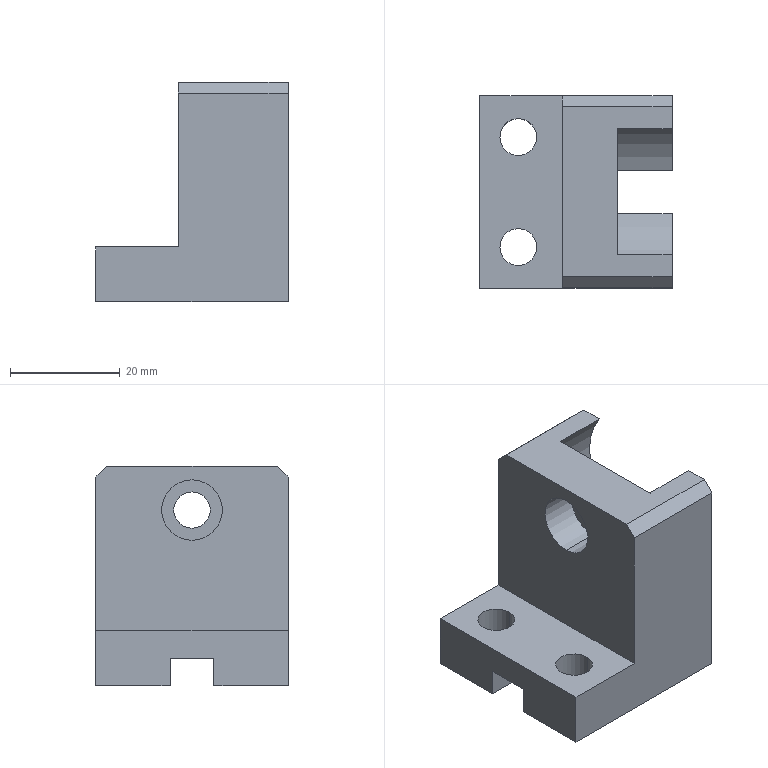Part | STEP file | Part 1^Dual platform unit | 1 solid | 27 faces | box 35 x 35 x 40 mm | volume 24064 mm3 | plane 17 | cylinder 10 | commonest cylinder face diameters 6.7 x4 6.6 x2 11 x2 28 x2
STEP:
#1=CARTESIAN_POINT('',(-416.35,-17.5,0.));
#2=VERTEX_POINT('',#1);
#3=CARTESIAN_POINT('',(-409.65,-17.5,0.));
#4=VERTEX_POINT('',#3);
#5=CARTESIAN_POINT('',(-413.,-17.5,0.));
#6=DIRECTION('',(0.,0.,1.));
#7=DIRECTION('',(1.,0.,0.));
#8=AXIS2_PLACEMENT_3D('',#5,#6,#7);
#9=CIRCLE('',#8,3.35);
#10=EDGE_CURVE('',#2,#4,#9,.T.);
#11=ORIENTED_EDGE('',*,*,#10,.F.);
#12=CARTESIAN_POINT('',(-416.35,-17.5,10.));
#13=VERTEX_POINT('',#12);
#14=CARTESIAN_POINT('',(-416.35,-17.5,10.));
#15=DIRECTION('',(0.,0.,1.));
#16=VECTOR('',#15,1000.);
#17=LINE('',#14,#16);
#18=EDGE_CURVE('',#2,#13,#17,.T.);
#19=ORIENTED_EDGE('',*,*,#18,.T.);
#20=CARTESIAN_POINT('',(-409.65,-17.5,10.));
#21=VERTEX_POINT('',#20);
#22=CARTESIAN_POINT('',(-413.,-17.5,10.));
#23=DIRECTION('',(0.,0.,1.));
#24=DIRECTION('',(1.,0.,0.));
#25=AXIS2_PLACEMENT_3D('',#22,#23,#24);
#26=CIRCLE('',#25,3.35);
#27=EDGE_CURVE('',#13,#21,#26,.T.);
#28=ORIENTED_EDGE('',*,*,#27,.T.);
#29=CARTESIAN_POINT('',(-409.65,-17.5,10.));
#30=DIRECTION('',(0.,0.,1.));
#31=VECTOR('',#30,1000.);
#32=LINE('',#29,#31);
#33=EDGE_CURVE('',#4,#21,#32,.T.);
#34=ORIENTED_EDGE('',*,*,#33,.F.);
#35=EDGE_LOOP('',(#11,#19,#28,#34));
#36=FACE_OUTER_BOUND('',#35,.T.);
#37=CARTESIAN_POINT('',(-413.,-17.5,10.));
#38=DIRECTION('',(0.,0.,1.));
#39=DIRECTION('',(1.,0.,0.));
#40=AXIS2_PLACEMENT_3D('',#37,#38,#39);
#41=CYLINDRICAL_SURFACE('',#40,3.35);
#42=ADVANCED_FACE('',(#36),#41,.F.);
#43=CARTESIAN_POINT('',(-416.35,-37.5,0.));
#44=VERTEX_POINT('',#43);
#45=CARTESIAN_POINT('',(-409.65,-37.5,0.));
#46=VERTEX_POINT('',#45);
#47=CARTESIAN_POINT('',(-413.,-37.5,0.));
#48=DIRECTION('',(0.,0.,1.));
#49=DIRECTION('',(1.,0.,0.));
#50=AXIS2_PLACEMENT_3D('',#47,#48,#49);
#51=CIRCLE('',#50,3.35);
#52=EDGE_CURVE('',#44,#46,#51,.T.);
#53=ORIENTED_EDGE('',*,*,#52,.F.);
#54=CARTESIAN_POINT('',(-416.35,-37.5,10.));
#55=VERTEX_POINT('',#54);
#56=CARTESIAN_POINT('',(-416.35,-37.5,10.));
#57=DIRECTION('',(0.,0.,1.));
#58=VECTOR('',#57,1000.);
#59=LINE('',#56,#58);
#60=EDGE_CURVE('',#44,#55,#59,.T.);
#61=ORIENTED_EDGE('',*,*,#60,.T.);
#62=CARTESIAN_POINT('',(-409.65,-37.5,10.));
#63=VERTEX_POINT('',#62);
#64=CARTESIAN_POINT('',(-413.,-37.5,10.));
#65=DIRECTION('',(0.,0.,1.));
#66=DIRECTION('',(1.,0.,0.));
#67=AXIS2_PLACEMENT_3D('',#64,#65,#66);
#68=CIRCLE('',#67,3.35);
#69=EDGE_CURVE('',#55,#63,#68,.T.);
#70=ORIENTED_EDGE('',*,*,#69,.T.);
#71=CARTESIAN_POINT('',(-409.65,-37.5,10.));
#72=DIRECTION('',(0.,0.,1.));
#73=VECTOR('',#72,1000.);
#74=LINE('',#71,#73);
#75=EDGE_CURVE('',#46,#63,#74,.T.);
#76=ORIENTED_EDGE('',*,*,#75,.F.);
#77=EDGE_LOOP('',(#53,#61,#70,#76));
#78=FACE_OUTER_BOUND('',#77,.T.);
#79=CARTESIAN_POINT('',(-413.,-37.5,10.));
#80=DIRECTION('',(0.,0.,1.));
#81=DIRECTION('',(1.,0.,0.));
#82=AXIS2_PLACEMENT_3D('',#79,#80,#81);
#83=CYLINDRICAL_SURFACE('',#82,3.35);
#84=ADVANCED_FACE('',(#78),#83,.F.);
#85=CARTESIAN_POINT('',(-398.2,-27.5,26.5));
#86=VERTEX_POINT('',#85);
#87=CARTESIAN_POINT('',(-398.2,-27.5,37.5));
#88=VERTEX_POINT('',#87);
#89=CARTESIAN_POINT('',(-398.2,-27.5,32.));
#90=DIRECTION('',(-1.,0.,0.));
#91=DIRECTION('',(0.,0.,1.));
#92=AXIS2_PLACEMENT_3D('',#89,#90,#91);
#93=CIRCLE('',#92,5.5);
#94=EDGE_CURVE('',#86,#88,#93,.T.);
#95=ORIENTED_EDGE('',*,*,#94,.F.);
#96=CARTESIAN_POINT('',(-405.,-27.5,26.5));
#97=VERTEX_POINT('',#96);
#98=CARTESIAN_POINT('',(-405.,-27.5,26.5));
#99=DIRECTION('',(-1.,0.,0.));
#100=VECTOR('',#99,1000.);
#101=LINE('',#98,#100);
#102=EDGE_CURVE('',#86,#97,#101,.T.);
#103=ORIENTED_EDGE('',*,*,#102,.T.);
#104=CARTESIAN_POINT('',(-405.,-27.5,37.5));
#105=VERTEX_POINT('',#104);
#106=CARTESIAN_POINT('',(-405.,-27.5,32.));
#107=DIRECTION('',(-1.,0.,0.));
#108=DIRECTION('',(0.,0.,1.));
#109=AXIS2_PLACEMENT_3D('',#106,#107,#108);
#110=CIRCLE('',#109,5.5);
#111=EDGE_CURVE('',#97,#105,#110,.T.);
#112=ORIENTED_EDGE('',*,*,#111,.T.);
#113=CARTESIAN_POINT('',(-405.,-27.5,37.5));
#114=DIRECTION('',(-1.,0.,0.));
#115=VECTOR('',#114,1000.);
#116=LINE('',#113,#115);
#117=EDGE_CURVE('',#88,#105,#116,.T.);
#118=ORIENTED_EDGE('',*,*,#117,.F.);
#119=EDGE_LOOP('',(#95,#103,#112,#118));
#120=FACE_OUTER_BOUND('',#119,.T.);
#121=CARTESIAN_POINT('',(-405.,-27.5,32.));
#122=DIRECTION('',(-1.,0.,0.));
#123=DIRECTION('',(0.,0.,1.));
#124=AXIS2_PLACEMENT_3D('',#121,#122,#123);
#125=CYLINDRICAL_SURFACE('',#124,5.5);
#126=ADVANCED_FACE('',(#120),#125,.F.);
#127=CARTESIAN_POINT('',(-395.,-27.5,35.3));
#128=VERTEX_POINT('',#127);
#129=CARTESIAN_POINT('',(-395.,-27.5,28.7));
#130=VERTEX_POINT('',#129);
#131=CARTESIAN_POINT('',(-395.,-27.5,32.));
#132=DIRECTION('',(1.,0.,0.));
#133=DIRECTION('',(0.,0.,-1.));
#134=AXIS2_PLACEMENT_3D('',#131,#132,#133);
#135=CIRCLE('',#134,3.3);
#136=EDGE_CURVE('',#128,#130,#135,.T.);
#137=ORIENTED_EDGE('',*,*,#136,.T.);
#138=CARTESIAN_POINT('',(-398.2,-27.5,28.7));
#139=VERTEX_POINT('',#138);
#140=CARTESIAN_POINT('',(-405.,-27.5,28.7));
#141=DIRECTION('',(-1.,0.,0.));
#142=VECTOR('',#141,1000.);
#143=LINE('',#140,#142);
#144=EDGE_CURVE('',#130,#139,#143,.T.);
#145=ORIENTED_EDGE('',*,*,#144,.T.);
#146=CARTESIAN_POINT('',(-398.2,-27.5,35.3));
#147=VERTEX_POINT('',#146);
#148=CARTESIAN_POINT('',(-398.2,-27.5,32.));
#149=DIRECTION('',(-1.,0.,0.));
#150=DIRECTION('',(0.,0.,1.));
#151=AXIS2_PLACEMENT_3D('',#148,#149,#150);
#152=CIRCLE('',#151,3.3);
#153=EDGE_CURVE('',#139,#147,#152,.T.);
#154=ORIENTED_EDGE('',*,*,#153,.T.);
#155=CARTESIAN_POINT('',(-405.,-27.5,35.3));
#156=DIRECTION('',(-1.,0.,0.));
#157=VECTOR('',#156,1000.);
#158=LINE('',#155,#157);
#159=EDGE_CURVE('',#128,#147,#158,.T.);
#160=ORIENTED_EDGE('',*,*,#159,.F.);
#161=EDGE_LOOP('',(#137,#145,#154,#160));
#162=FACE_OUTER_BOUND('',#161,.T.);
#163=CARTESIAN_POINT('',(-405.,-27.5,32.));
#164=DIRECTION('',(-1.,0.,0.));
#165=DIRECTION('',(0.,0.,1.));
#166=AXIS2_PLACEMENT_3D('',#163,#164,#165);
#167=CYLINDRICAL_SURFACE('',#166,3.3);
#168=ADVANCED_FACE('',(#162),#167,.F.);
#169=CARTESIAN_POINT('',(-413.,-37.5,0.));
#170=DIRECTION('',(0.,0.,1.));
#171=DIRECTION('',(1.,0.,0.));
#172=AXIS2_PLACEMENT_3D('',#169,#170,#171);
#173=CIRCLE('',#172,3.35);
#174=EDGE_CURVE('',#46,#44,#173,.T.);
#175=ORIENTED_EDGE('',*,*,#174,.T.);
#176=ORIENTED_EDGE('',*,*,#52,.T.);
#177=EDGE_LOOP('',(#175,#176));
#178=FACE_BOUND('',#177,.T.);
#179=CARTESIAN_POINT('',(-420.,-31.5,0.));
#180=VERTEX_POINT('',#179);
#181=CARTESIAN_POINT('',(-420.,-45.,0.));
#182=VERTEX_POINT('',#181);
#183=CARTESIAN_POINT('',(-420.,-45.,0.));
#184=DIRECTION('',(0.,-1.,0.));
#185=VECTOR('',#184,1000.);
#186=LINE('',#183,#185);
#187=EDGE_CURVE('',#180,#182,#186,.T.);
#188=ORIENTED_EDGE('',*,*,#187,.F.);
#189=CARTESIAN_POINT('',(-385.,-31.5,0.));
#190=VERTEX_POINT('',#189);
#191=CARTESIAN_POINT('',(-395.,-31.5,0.));
#192=DIRECTION('',(1.,0.,0.));
#193=VECTOR('',#192,1000.);
#194=LINE('',#191,#193);
#195=EDGE_CURVE('',#180,#190,#194,.T.);
#196=ORIENTED_EDGE('',*,*,#195,.T.);
#197=CARTESIAN_POINT('',(-385.,-45.,0.));
#198=VERTEX_POINT('',#197);
#199=CARTESIAN_POINT('',(-385.,-45.,0.));
#200=DIRECTION('',(0.,1.,0.));
#201=VECTOR('',#200,1000.);
#202=LINE('',#199,#201);
#203=EDGE_CURVE('',#198,#190,#202,.T.);
#204=ORIENTED_EDGE('',*,*,#203,.F.);
#205=CARTESIAN_POINT('',(-385.,-45.,0.));
#206=DIRECTION('',(1.,0.,0.));
#207=VECTOR('',#206,1000.);
#208=LINE('',#205,#207);
#209=EDGE_CURVE('',#182,#198,#208,.T.);
#210=ORIENTED_EDGE('',*,*,#209,.F.);
#211=EDGE_LOOP('',(#188,#196,#204,#210));
#212=FACE_OUTER_BOUND('',#211,.T.);
#213=CARTESIAN_POINT('',(0.,0.,0.));
#214=DIRECTION('',(0.,0.,1.));
#215=DIRECTION('',(1.,0.,0.));
#216=AXIS2_PLACEMENT_3D('',#213,#214,#215);
#217=PLANE('',#216);
#218=ADVANCED_FACE('',(#178,#212),#217,.F.);
#219=CARTESIAN_POINT('',(-385.,-43.,40.));
#220=VERTEX_POINT('',#219);
#221=CARTESIAN_POINT('',(-385.,-38.989,40.));
#222=VERTEX_POINT('',#221);
#223=CARTESIAN_POINT('',(-385.,-45.,40.));
#224=DIRECTION('',(0.,1.,0.));
#225=VECTOR('',#224,1000.);
#226=LINE('',#223,#225);
#227=EDGE_CURVE('',#220,#222,#226,.T.);
#228=ORIENTED_EDGE('',*,*,#227,.F.);
#229=CARTESIAN_POINT('',(-385.,-45.,38.));
#230=VERTEX_POINT('',#229);
#231=CARTESIAN_POINT('',(-385.,-43.,40.));
#232=DIRECTION('',(0.,-0.7071,-0.7071));
#233=VECTOR('',#232,1000.);
#234=LINE('',#231,#233);
#235=EDGE_CURVE('',#220,#230,#234,.T.);
#236=ORIENTED_EDGE('',*,*,#235,.T.);
#237=CARTESIAN_POINT('',(-385.,-45.,40.));
#238=DIRECTION('',(0.,0.,-1.));
#239=VECTOR('',#238,1000.);
#240=LINE('',#237,#239);
#241=EDGE_CURVE('',#230,#198,#240,.T.);
#242=ORIENTED_EDGE('',*,*,#241,.T.);
#243=ORIENTED_EDGE('',*,*,#203,.T.);
#244=CARTESIAN_POINT('',(-385.,-31.5,18.584));
#245=VERTEX_POINT('',#244);
#246=CARTESIAN_POINT('',(-385.,-31.5,0.));
#247=DIRECTION('',(0.,0.,-1.));
#248=VECTOR('',#247,1000.);
#249=LINE('',#246,#248);
#250=EDGE_CURVE('',#245,#190,#249,.T.);
#251=ORIENTED_EDGE('',*,*,#250,.F.);
#252=CARTESIAN_POINT('',(-385.,-27.5,32.));
#253=DIRECTION('',(1.,0.,0.));
#254=DIRECTION('',(0.,0.,-1.));
#255=AXIS2_PLACEMENT_3D('',#252,#253,#254);
#256=CIRCLE('',#255,14.);
#257=EDGE_CURVE('',#222,#245,#256,.T.);
#258=ORIENTED_EDGE('',*,*,#257,.F.);
#259=EDGE_LOOP('',(#228,#236,#242,#243,#251,#258));
#260=FACE_OUTER_BOUND('',#259,.T.);
#261=CARTESIAN_POINT('',(-385.,-45.,40.));
#262=DIRECTION('',(-1.,0.,0.));
#263=DIRECTION('',(0.,0.,1.));
#264=AXIS2_PLACEMENT_3D('',#261,#262,#263);
#265=PLANE('',#264);
#266=ADVANCED_FACE('',(#260),#265,.F.);
#267=ORIENTED_EDGE('',*,*,#257,.T.);
#268=CARTESIAN_POINT('',(-395.,-31.5,18.584));
#269=VERTEX_POINT('',#268);
#270=CARTESIAN_POINT('',(-395.,-31.5,18.584));
#271=DIRECTION('',(-1.,0.,0.));
#272=VECTOR('',#271,1000.);
#273=LINE('',#270,#272);
#274=EDGE_CURVE('',#245,#269,#273,.T.);
#275=ORIENTED_EDGE('',*,*,#274,.T.);
#276=CARTESIAN_POINT('',(-395.,-38.989,40.));
#277=VERTEX_POINT('',#276);
#278=CARTESIAN_POINT('',(-395.,-27.5,32.));
#279=DIRECTION('',(1.,0.,0.));
#280=DIRECTION('',(0.,0.,-1.));
#281=AXIS2_PLACEMENT_3D('',#278,#279,#280);
#282=CIRCLE('',#281,14.);
#283=EDGE_CURVE('',#277,#269,#282,.T.);
#284=ORIENTED_EDGE('',*,*,#283,.F.);
#285=CARTESIAN_POINT('',(-395.,-38.989,40.));
#286=DIRECTION('',(1.,0.,0.));
#287=VECTOR('',#286,1000.);
#288=LINE('',#285,#287);
#289=EDGE_CURVE('',#277,#222,#288,.T.);
#290=ORIENTED_EDGE('',*,*,#289,.T.);
#291=EDGE_LOOP('',(#267,#275,#284,#290));
#292=FACE_OUTER_BOUND('',#291,.T.);
#293=CARTESIAN_POINT('',(-395.,-27.5,32.));
#294=DIRECTION('',(1.,0.,0.));
#295=DIRECTION('',(0.,0.,-1.));
#296=AXIS2_PLACEMENT_3D('',#293,#294,#295);
#297=CYLINDRICAL_SURFACE('',#296,14.);
#298=ADVANCED_FACE('',(#292),#297,.F.);
#299=CARTESIAN_POINT('',(-385.,-10.,38.));
#300=VERTEX_POINT('',#299);
#301=CARTESIAN_POINT('',(-385.,-10.,0.));
#302=VERTEX_POINT('',#301);
#303=CARTESIAN_POINT('',(-385.,-10.,40.));
#304=DIRECTION('',(0.,0.,-1.));
#305=VECTOR('',#304,1000.);
#306=LINE('',#303,#305);
#307=EDGE_CURVE('',#300,#302,#306,.T.);
#308=ORIENTED_EDGE('',*,*,#307,.F.);
#309=CARTESIAN_POINT('',(-385.,-12.,40.));
#310=VERTEX_POINT('',#309);
#311=CARTESIAN_POINT('',(-385.,-12.,40.));
#312=DIRECTION('',(0.,-0.7071,0.7071));
#313=VECTOR('',#312,1000.);
#314=LINE('',#311,#313);
#315=EDGE_CURVE('',#300,#310,#314,.T.);
#316=ORIENTED_EDGE('',*,*,#315,.T.);
#317=CARTESIAN_POINT('',(-385.,-16.011,40.));
#318=VERTEX_POINT('',#317);
#319=CARTESIAN_POINT('',(-385.,-45.,40.));
#320=DIRECTION('',(0.,1.,0.));
#321=VECTOR('',#320,1000.);
#322=LINE('',#319,#321);
#323=EDGE_CURVE('',#318,#310,#322,.T.);
#324=ORIENTED_EDGE('',*,*,#323,.F.);
#325=CARTESIAN_POINT('',(-385.,-23.5,18.584));
#326=VERTEX_POINT('',#325);
#327=CARTESIAN_POINT('',(-385.,-27.5,32.));
#328=DIRECTION('',(1.,0.,0.));
#329=DIRECTION('',(0.,0.,-1.));
#330=AXIS2_PLACEMENT_3D('',#327,#328,#329);
#331=CIRCLE('',#330,14.);
#332=EDGE_CURVE('',#326,#318,#331,.T.);
#333=ORIENTED_EDGE('',*,*,#332,.F.);
#334=CARTESIAN_POINT('',(-385.,-23.5,0.));
#335=VERTEX_POINT('',#334);
#336=CARTESIAN_POINT('',(-385.,-23.5,0.));
#337=DIRECTION('',(0.,0.,1.));
#338=VECTOR('',#337,1000.);
#339=LINE('',#336,#338);
#340=EDGE_CURVE('',#335,#326,#339,.T.);
#341=ORIENTED_EDGE('',*,*,#340,.F.);
#342=CARTESIAN_POINT('',(-385.,-45.,0.));
#343=DIRECTION('',(0.,1.,0.));
#344=VECTOR('',#343,1000.);
#345=LINE('',#342,#344);
#346=EDGE_CURVE('',#335,#302,#345,.T.);
#347=ORIENTED_EDGE('',*,*,#346,.T.);
#348=EDGE_LOOP('',(#308,#316,#324,#333,#341,#347));
#349=FACE_OUTER_BOUND('',#348,.T.);
#350=CARTESIAN_POINT('',(-385.,-45.,40.));
#351=DIRECTION('',(-1.,0.,0.));
#352=DIRECTION('',(0.,0.,1.));
#353=AXIS2_PLACEMENT_3D('',#350,#351,#352);
#354=PLANE('',#353);
#355=ADVANCED_FACE('',(#349),#354,.F.);
#356=CARTESIAN_POINT('',(-405.,-10.,38.));
#357=VERTEX_POINT('',#356);
#358=CARTESIAN_POINT('',(-405.,-10.,10.));
#359=VERTEX_POINT('',#358);
#360=CARTESIAN_POINT('',(-405.,-10.,40.));
#361=DIRECTION('',(0.,0.,-1.));
#362=VECTOR('',#361,1000.);
#363=LINE('',#360,#362);
#364=EDGE_CURVE('',#357,#359,#363,.T.);
#365=ORIENTED_EDGE('',*,*,#364,.F.);
#366=CARTESIAN_POINT('',(-385.,-10.,38.));
#367=DIRECTION('',(1.,0.,0.));
#368=VECTOR('',#367,1000.);
#369=LINE('',#366,#368);
#370=EDGE_CURVE('',#357,#300,#369,.T.);
#371=ORIENTED_EDGE('',*,*,#370,.T.);
#372=ORIENTED_EDGE('',*,*,#307,.T.);
#373=CARTESIAN_POINT('',(-420.,-10.,0.));
#374=VERTEX_POINT('',#373);
#375=CARTESIAN_POINT('',(-385.,-10.,0.));
#376=DIRECTION('',(-1.,0.,0.));
#377=VECTOR('',#376,1000.);
#378=LINE('',#375,#377);
#379=EDGE_CURVE('',#302,#374,#378,.T.);
#380=ORIENTED_EDGE('',*,*,#379,.T.);
#381=CARTESIAN_POINT('',(-420.,-10.,10.));
#382=VERTEX_POINT('',#381);
#383=CARTESIAN_POINT('',(-420.,-10.,40.));
#384=DIRECTION('',(0.,0.,-1.));
#385=VECTOR('',#384,1000.);
#386=LINE('',#383,#385);
#387=EDGE_CURVE('',#382,#374,#386,.T.);
#388=ORIENTED_EDGE('',*,*,#387,.F.);
#389=CARTESIAN_POINT('',(-405.,-10.,10.));
#390=DIRECTION('',(-1.,0.,0.));
#391=VECTOR('',#390,1000.);
#392=LINE('',#389,#391);
#393=EDGE_CURVE('',#359,#382,#392,.T.);
#394=ORIENTED_EDGE('',*,*,#393,.F.);
#395=EDGE_LOOP('',(#365,#371,#372,#380,#388,#394));
#396=FACE_OUTER_BOUND('',#395,.T.);
#397=CARTESIAN_POINT('',(-385.,-10.,40.));
#398=DIRECTION('',(0.,-1.,0.));
#399=DIRECTION('',(1.,0.,0.));
#400=AXIS2_PLACEMENT_3D('',#397,#398,#399);
#401=PLANE('',#400);
#402=ADVANCED_FACE('',(#396),#401,.F.);
#403=CARTESIAN_POINT('',(-420.,-31.5,5.));
#404=VERTEX_POINT('',#403);
#405=CARTESIAN_POINT('',(-420.,-23.5,5.));
#406=VERTEX_POINT('',#405);
#407=CARTESIAN_POINT('',(-420.,-23.5,5.));
#408=DIRECTION('',(0.,1.,0.));
#409=VECTOR('',#408,1000.);
#410=LINE('',#407,#409);
#411=EDGE_CURVE('',#404,#406,#410,.T.);
#412=ORIENTED_EDGE('',*,*,#411,.F.);
#413=CARTESIAN_POINT('',(-420.,-31.5,5.));
#414=DIRECTION('',(0.,0.,-1.));
#415=VECTOR('',#414,1000.);
#416=LINE('',#413,#415);
#417=EDGE_CURVE('',#404,#180,#416,.T.);
#418=ORIENTED_EDGE('',*,*,#417,.T.);
#419=ORIENTED_EDGE('',*,*,#187,.T.);
#420=CARTESIAN_POINT('',(-420.,-45.,10.));
#421=VERTEX_POINT('',#420);
#422=CARTESIAN_POINT('',(-420.,-45.,40.));
#423=DIRECTION('',(0.,0.,-1.));
#424=VECTOR('',#423,1000.);
#425=LINE('',#422,#424);
#426=EDGE_CURVE('',#421,#182,#425,.T.);
#427=ORIENTED_EDGE('',*,*,#426,.F.);
#428=CARTESIAN_POINT('',(-420.,-10.,10.));
#429=DIRECTION('',(0.,-1.,0.));
#430=VECTOR('',#429,1000.);
#431=LINE('',#428,#430);
#432=EDGE_CURVE('',#382,#421,#431,.T.);
#433=ORIENTED_EDGE('',*,*,#432,.F.);
#434=ORIENTED_EDGE('',*,*,#387,.T.);
#435=CARTESIAN_POINT('',(-420.,-23.5,0.));
#436=VERTEX_POINT('',#435);
#437=CARTESIAN_POINT('',(-420.,-45.,0.));
#438=DIRECTION('',(0.,-1.,0.));
#439=VECTOR('',#438,1000.);
#440=LINE('',#437,#439);
#441=EDGE_CURVE('',#374,#436,#440,.T.);
#442=ORIENTED_EDGE('',*,*,#441,.T.);
#443=CARTESIAN_POINT('',(-420.,-23.5,5.));
#444=DIRECTION('',(0.,0.,-1.));
#445=VECTOR('',#444,1000.);
#446=LINE('',#443,#445);
#447=EDGE_CURVE('',#406,#436,#446,.T.);
#448=ORIENTED_EDGE('',*,*,#447,.F.);
#449=EDGE_LOOP('',(#412,#418,#419,#427,#433,#434,#442,#448));
#450=FACE_OUTER_BOUND('',#449,.T.);
#451=CARTESIAN_POINT('',(-420.,-45.,40.));
#452=DIRECTION('',(1.,0.,0.));
#453=DIRECTION('',(0.,0.,-1.));
#454=AXIS2_PLACEMENT_3D('',#451,#452,#453);
#455=PLANE('',#454);
#456=ADVANCED_FACE('',(#450),#455,.F.);
#457=ORIENTED_EDGE('',*,*,#241,.F.);
#458=CARTESIAN_POINT('',(-405.,-45.,38.));
#459=VERTEX_POINT('',#458);
#460=CARTESIAN_POINT('',(-405.,-45.,38.));
#461=DIRECTION('',(-1.,0.,0.));
#462=VECTOR('',#461,1000.);
#463=LINE('',#460,#462);
#464=EDGE_CURVE('',#230,#459,#463,.T.);
#465=ORIENTED_EDGE('',*,*,#464,.T.);
#466=CARTESIAN_POINT('',(-405.,-45.,10.));
#467=VERTEX_POINT('',#466);
#468=CARTESIAN_POINT('',(-405.,-45.,40.));
#469=DIRECTION('',(0.,0.,1.));
#470=VECTOR('',#469,1000.);
#471=LINE('',#468,#470);
#472=EDGE_CURVE('',#467,#459,#471,.T.);
#473=ORIENTED_EDGE('',*,*,#472,.F.);
#474=CARTESIAN_POINT('',(-405.,-45.,10.));
#475=DIRECTION('',(-1.,0.,0.));
#476=VECTOR('',#475,1000.);
#477=LINE('',#474,#476);
#478=EDGE_CURVE('',#467,#421,#477,.T.);
#479=ORIENTED_EDGE('',*,*,#478,.T.);
#480=ORIENTED_EDGE('',*,*,#426,.T.);
#481=ORIENTED_EDGE('',*,*,#209,.T.);
#482=EDGE_LOOP('',(#457,#465,#473,#479,#480,#481));
#483=FACE_OUTER_BOUND('',#482,.T.);
#484=CARTESIAN_POINT('',(-385.,-45.,40.));
#485=DIRECTION('',(0.,1.,0.));
#486=DIRECTION('',(0.,0.,1.));
#487=AXIS2_PLACEMENT_3D('',#484,#485,#486);
#488=PLANE('',#487);
#489=ADVANCED_FACE('',(#483),#488,.F.);
#490=ORIENTED_EDGE('',*,*,#323,.T.);
#491=CARTESIAN_POINT('',(-405.,-12.,40.));
#492=VERTEX_POINT('',#491);
#493=CARTESIAN_POINT('',(-405.,-12.,40.));
#494=DIRECTION('',(-1.,0.,0.));
#495=VECTOR('',#494,1000.);
#496=LINE('',#493,#495);
#497=EDGE_CURVE('',#310,#492,#496,.T.);
#498=ORIENTED_EDGE('',*,*,#497,.T.);
#499=CARTESIAN_POINT('',(-405.,-43.,40.));
#500=VERTEX_POINT('',#499);
#501=CARTESIAN_POINT('',(-405.,-10.,40.));
#502=DIRECTION('',(0.,1.,0.));
#503=VECTOR('',#502,1000.);
#504=LINE('',#501,#503);
#505=EDGE_CURVE('',#500,#492,#504,.T.);
#506=ORIENTED_EDGE('',*,*,#505,.F.);
#507=CARTESIAN_POINT('',(-385.,-43.,40.));
#508=DIRECTION('',(1.,0.,0.));
#509=VECTOR('',#508,1000.);
#510=LINE('',#507,#509);
#511=EDGE_CURVE('',#500,#220,#510,.T.);
#512=ORIENTED_EDGE('',*,*,#511,.T.);
#513=ORIENTED_EDGE('',*,*,#227,.T.);
#514=ORIENTED_EDGE('',*,*,#289,.F.);
#515=CARTESIAN_POINT('',(-395.,-16.011,40.));
#516=VERTEX_POINT('',#515);
#517=CARTESIAN_POINT('',(-395.,0.,40.));
#518=DIRECTION('',(0.,1.,0.));
#519=VECTOR('',#518,1000.);
#520=LINE('',#517,#519);
#521=EDGE_CURVE('',#277,#516,#520,.T.);
#522=ORIENTED_EDGE('',*,*,#521,.T.);
#523=CARTESIAN_POINT('',(-395.,-16.011,40.));
#524=DIRECTION('',(-1.,0.,0.));
#525=VECTOR('',#524,1000.);
#526=LINE('',#523,#525);
#527=EDGE_CURVE('',#318,#516,#526,.T.);
#528=ORIENTED_EDGE('',*,*,#527,.F.);
#529=EDGE_LOOP('',(#490,#498,#506,#512,#513,#514,#522,#528));
#530=FACE_OUTER_BOUND('',#529,.T.);
#531=CARTESIAN_POINT('',(0.,0.,40.));
#532=DIRECTION('',(0.,0.,1.));
#533=DIRECTION('',(1.,0.,0.));
#534=AXIS2_PLACEMENT_3D('',#531,#532,#533);
#535=PLANE('',#534);
#536=ADVANCED_FACE('',(#530),#535,.T.);
#537=CARTESIAN_POINT('',(-413.,-17.5,0.));
#538=DIRECTION('',(0.,0.,1.));
#539=DIRECTION('',(1.,0.,0.));
#540=AXIS2_PLACEMENT_3D('',#537,#538,#539);
#541=CIRCLE('',#540,3.35);
#542=EDGE_CURVE('',#4,#2,#541,.T.);
#543=ORIENTED_EDGE('',*,*,#542,.T.);
#544=ORIENTED_EDGE('',*,*,#10,.T.);
#545=EDGE_LOOP('',(#543,#544));
#546=FACE_BOUND('',#545,.T.);
#547=CARTESIAN_POINT('',(-395.,-23.5,0.));
#548=DIRECTION('',(1.,0.,0.));
#549=VECTOR('',#548,1000.);
#550=LINE('',#547,#549);
#551=EDGE_CURVE('',#436,#335,#550,.T.);
#552=ORIENTED_EDGE('',*,*,#551,.F.);
#553=ORIENTED_EDGE('',*,*,#441,.F.);
#554=ORIENTED_EDGE('',*,*,#379,.F.);
#555=ORIENTED_EDGE('',*,*,#346,.F.);
#556=EDGE_LOOP('',(#552,#553,#554,#555));
#557=FACE_OUTER_BOUND('',#556,.T.);
#558=CARTESIAN_POINT('',(0.,0.,0.));
#559=DIRECTION('',(0.,0.,1.));
#560=DIRECTION('',(1.,0.,0.));
#561=AXIS2_PLACEMENT_3D('',#558,#559,#560);
#562=PLANE('',#561);
#563=ADVANCED_FACE('',(#546,#557),#562,.F.);
#564=CARTESIAN_POINT('',(-413.,-17.5,10.));
#565=DIRECTION('',(0.,0.,1.));
#566=DIRECTION('',(1.,0.,0.));
#567=AXIS2_PLACEMENT_3D('',#564,#565,#566);
#568=CIRCLE('',#567,3.35);
#569=EDGE_CURVE('',#21,#13,#568,.T.);
#570=ORIENTED_EDGE('',*,*,#569,.F.);
#571=ORIENTED_EDGE('',*,*,#27,.F.);
#572=EDGE_LOOP('',(#570,#571));
#573=FACE_BOUND('',#572,.T.);
#574=CARTESIAN_POINT('',(-413.,-37.5,10.));
#575=DIRECTION('',(0.,0.,1.));
#576=DIRECTION('',(1.,0.,0.));
#577=AXIS2_PLACEMENT_3D('',#574,#575,#576);
#578=CIRCLE('',#577,3.35);
#579=EDGE_CURVE('',#63,#55,#578,.T.);
#580=ORIENTED_EDGE('',*,*,#579,.F.);
#581=ORIENTED_EDGE('',*,*,#69,.F.);
#582=EDGE_LOOP('',(#580,#581));
#583=FACE_BOUND('',#582,.T.);
#584=ORIENTED_EDGE('',*,*,#432,.T.);
#585=ORIENTED_EDGE('',*,*,#478,.F.);
#586=CARTESIAN_POINT('',(-405.,-10.,10.));
#587=DIRECTION('',(0.,-1.,0.));
#588=VECTOR('',#587,1000.);
#589=LINE('',#586,#588);
#590=EDGE_CURVE('',#359,#467,#589,.T.);
#591=ORIENTED_EDGE('',*,*,#590,.F.);
#592=ORIENTED_EDGE('',*,*,#393,.T.);
#593=EDGE_LOOP('',(#584,#585,#591,#592));
#594=FACE_OUTER_BOUND('',#593,.T.);
#595=CARTESIAN_POINT('',(-405.,-10.,10.));
#596=DIRECTION('',(0.,0.,-1.));
#597=DIRECTION('',(0.,1.,0.));
#598=AXIS2_PLACEMENT_3D('',#595,#596,#597);
#599=PLANE('',#598);
#600=ADVANCED_FACE('',(#573,#583,#594),#599,.F.);
#601=CARTESIAN_POINT('',(-405.,-27.5,32.));
#602=DIRECTION('',(-1.,0.,0.));
#603=DIRECTION('',(0.,0.,1.));
#604=AXIS2_PLACEMENT_3D('',#601,#602,#603);
#605=CIRCLE('',#604,5.5);
#606=EDGE_CURVE('',#105,#97,#605,.T.);
#607=ORIENTED_EDGE('',*,*,#606,.F.);
#608=ORIENTED_EDGE('',*,*,#111,.F.);
#609=EDGE_LOOP('',(#607,#608));
#610=FACE_BOUND('',#609,.T.);
#611=ORIENTED_EDGE('',*,*,#505,.T.);
#612=CARTESIAN_POINT('',(-405.,-12.,40.));
#613=DIRECTION('',(0.,0.7071,-0.7071));
#614=VECTOR('',#613,1000.);
#615=LINE('',#612,#614);
#616=EDGE_CURVE('',#492,#357,#615,.T.);
#617=ORIENTED_EDGE('',*,*,#616,.T.);
#618=ORIENTED_EDGE('',*,*,#364,.T.);
#619=ORIENTED_EDGE('',*,*,#590,.T.);
#620=ORIENTED_EDGE('',*,*,#472,.T.);
#621=CARTESIAN_POINT('',(-405.,-43.,40.));
#622=DIRECTION('',(0.,0.7071,0.7071));
#623=VECTOR('',#622,1000.);
#624=LINE('',#621,#623);
#625=EDGE_CURVE('',#459,#500,#624,.T.);
#626=ORIENTED_EDGE('',*,*,#625,.T.);
#627=EDGE_LOOP('',(#611,#617,#618,#619,#620,#626));
#628=FACE_OUTER_BOUND('',#627,.T.);
#629=CARTESIAN_POINT('',(-405.,0.,0.));
#630=DIRECTION('',(1.,0.,0.));
#631=DIRECTION('',(0.,0.,-1.));
#632=AXIS2_PLACEMENT_3D('',#629,#630,#631);
#633=PLANE('',#632);
#634=ADVANCED_FACE('',(#610,#628),#633,.F.);
#635=CARTESIAN_POINT('',(-395.,-23.5,18.584));
#636=VERTEX_POINT('',#635);
#637=CARTESIAN_POINT('',(-395.,-27.5,32.));
#638=DIRECTION('',(1.,0.,0.));
#639=DIRECTION('',(0.,0.,-1.));
#640=AXIS2_PLACEMENT_3D('',#637,#638,#639);
#641=CIRCLE('',#640,14.);
#642=EDGE_CURVE('',#636,#516,#641,.T.);
#643=ORIENTED_EDGE('',*,*,#642,.F.);
#644=CARTESIAN_POINT('',(-395.,-23.5,18.584));
#645=DIRECTION('',(1.,0.,0.));
#646=VECTOR('',#645,1000.);
#647=LINE('',#644,#646);
#648=EDGE_CURVE('',#636,#326,#647,.T.);
#649=ORIENTED_EDGE('',*,*,#648,.T.);
#650=ORIENTED_EDGE('',*,*,#332,.T.);
#651=ORIENTED_EDGE('',*,*,#527,.T.);
#652=EDGE_LOOP('',(#643,#649,#650,#651));
#653=FACE_OUTER_BOUND('',#652,.T.);
#654=CARTESIAN_POINT('',(-395.,-27.5,32.));
#655=DIRECTION('',(1.,0.,0.));
#656=DIRECTION('',(0.,0.,-1.));
#657=AXIS2_PLACEMENT_3D('',#654,#655,#656);
#658=CYLINDRICAL_SURFACE('',#657,14.);
#659=ADVANCED_FACE('',(#653),#658,.F.);
#660=ORIENTED_EDGE('',*,*,#136,.F.);
#661=CARTESIAN_POINT('',(-395.,-27.5,32.));
#662=DIRECTION('',(1.,0.,0.));
#663=DIRECTION('',(0.,0.,-1.));
#664=AXIS2_PLACEMENT_3D('',#661,#662,#663);
#665=CIRCLE('',#664,3.3);
#666=EDGE_CURVE('',#130,#128,#665,.T.);
#667=ORIENTED_EDGE('',*,*,#666,.F.);
#668=EDGE_LOOP('',(#660,#667));
#669=FACE_BOUND('',#668,.T.);
#670=CARTESIAN_POINT('',(-395.,-23.5,5.));
#671=VERTEX_POINT('',#670);
#672=CARTESIAN_POINT('',(-395.,-31.5,5.));
#673=VERTEX_POINT('',#672);
#674=CARTESIAN_POINT('',(-395.,-27.5,5.));
#675=DIRECTION('',(0.,-1.,0.));
#676=VECTOR('',#675,1000.);
#677=LINE('',#674,#676);
#678=EDGE_CURVE('',#671,#673,#677,.T.);
#679=ORIENTED_EDGE('',*,*,#678,.F.);
#680=CARTESIAN_POINT('',(-395.,-23.5,0.));
#681=DIRECTION('',(0.,0.,1.));
#682=VECTOR('',#681,1000.);
#683=LINE('',#680,#682);
#684=EDGE_CURVE('',#671,#636,#683,.T.);
#685=ORIENTED_EDGE('',*,*,#684,.T.);
#686=ORIENTED_EDGE('',*,*,#642,.T.);
#687=ORIENTED_EDGE('',*,*,#521,.F.);
#688=ORIENTED_EDGE('',*,*,#283,.T.);
#689=CARTESIAN_POINT('',(-395.,-31.5,0.));
#690=DIRECTION('',(0.,0.,-1.));
#691=VECTOR('',#690,1000.);
#692=LINE('',#689,#691);
#693=EDGE_CURVE('',#269,#673,#692,.T.);
#694=ORIENTED_EDGE('',*,*,#693,.T.);
#695=EDGE_LOOP('',(#679,#685,#686,#687,#688,#694));
#696=FACE_OUTER_BOUND('',#695,.T.);
#697=CARTESIAN_POINT('',(-395.,-27.5,32.));
#698=DIRECTION('',(1.,0.,0.));
#699=DIRECTION('',(0.,0.,-1.));
#700=AXIS2_PLACEMENT_3D('',#697,#698,#699);
#701=PLANE('',#700);
#702=ADVANCED_FACE('',(#669,#696),#701,.T.);
#703=ORIENTED_EDGE('',*,*,#250,.T.);
#704=ORIENTED_EDGE('',*,*,#195,.F.);
#705=ORIENTED_EDGE('',*,*,#417,.F.);
#706=CARTESIAN_POINT('',(-420.,-31.5,5.));
#707=DIRECTION('',(-1.,0.,0.));
#708=VECTOR('',#707,1000.);
#709=LINE('',#706,#708);
#710=EDGE_CURVE('',#673,#404,#709,.T.);
#711=ORIENTED_EDGE('',*,*,#710,.F.);
#712=ORIENTED_EDGE('',*,*,#693,.F.);
#713=ORIENTED_EDGE('',*,*,#274,.F.);
#714=EDGE_LOOP('',(#703,#704,#705,#711,#712,#713));
#715=FACE_OUTER_BOUND('',#714,.T.);
#716=CARTESIAN_POINT('',(-395.,-31.5,0.));
#717=DIRECTION('',(0.,-1.,0.));
#718=DIRECTION('',(0.,0.,-1.));
#719=AXIS2_PLACEMENT_3D('',#716,#717,#718);
#720=PLANE('',#719);
#721=ADVANCED_FACE('',(#715),#720,.F.);
#722=ORIENTED_EDGE('',*,*,#684,.F.);
#723=CARTESIAN_POINT('',(-420.,-23.5,5.));
#724=DIRECTION('',(1.,0.,0.));
#725=VECTOR('',#724,1000.);
#726=LINE('',#723,#725);
#727=EDGE_CURVE('',#406,#671,#726,.T.);
#728=ORIENTED_EDGE('',*,*,#727,.F.);
#729=ORIENTED_EDGE('',*,*,#447,.T.);
#730=ORIENTED_EDGE('',*,*,#551,.T.);
#731=ORIENTED_EDGE('',*,*,#340,.T.);
#732=ORIENTED_EDGE('',*,*,#648,.F.);
#733=EDGE_LOOP('',(#722,#728,#729,#730,#731,#732));
#734=FACE_OUTER_BOUND('',#733,.T.);
#735=CARTESIAN_POINT('',(-395.,-23.5,0.));
#736=DIRECTION('',(0.,1.,0.));
#737=DIRECTION('',(0.,0.,1.));
#738=AXIS2_PLACEMENT_3D('',#735,#736,#737);
#739=PLANE('',#738);
#740=ADVANCED_FACE('',(#734),#739,.F.);
#741=ORIENTED_EDGE('',*,*,#678,.T.);
#742=ORIENTED_EDGE('',*,*,#710,.T.);
#743=ORIENTED_EDGE('',*,*,#411,.T.);
#744=ORIENTED_EDGE('',*,*,#727,.T.);
#745=EDGE_LOOP('',(#741,#742,#743,#744));
#746=FACE_OUTER_BOUND('',#745,.T.);
#747=CARTESIAN_POINT('',(0.,0.,5.));
#748=DIRECTION('',(0.,0.,1.));
#749=DIRECTION('',(1.,0.,0.));
#750=AXIS2_PLACEMENT_3D('',#747,#748,#749);
#751=PLANE('',#750);
#752=ADVANCED_FACE('',(#746),#751,.F.);
#753=ORIENTED_EDGE('',*,*,#315,.F.);
#754=ORIENTED_EDGE('',*,*,#370,.F.);
#755=ORIENTED_EDGE('',*,*,#616,.F.);
#756=ORIENTED_EDGE('',*,*,#497,.F.);
#757=EDGE_LOOP('',(#753,#754,#755,#756));
#758=FACE_OUTER_BOUND('',#757,.T.);
#759=CARTESIAN_POINT('',(0.,-12.,40.));
#760=DIRECTION('',(0.,0.7071,0.7071));
#761=DIRECTION('',(1.,0.,0.));
#762=AXIS2_PLACEMENT_3D('',#759,#760,#761);
#763=PLANE('',#762);
#764=ADVANCED_FACE('',(#758),#763,.T.);
#765=ORIENTED_EDGE('',*,*,#625,.F.);
#766=ORIENTED_EDGE('',*,*,#464,.F.);
#767=ORIENTED_EDGE('',*,*,#235,.F.);
#768=ORIENTED_EDGE('',*,*,#511,.F.);
#769=EDGE_LOOP('',(#765,#766,#767,#768));
#770=FACE_OUTER_BOUND('',#769,.T.);
#771=CARTESIAN_POINT('',(0.,-43.,40.));
#772=DIRECTION('',(0.,-0.7071,0.7071));
#773=DIRECTION('',(-1.,0.,0.));
#774=AXIS2_PLACEMENT_3D('',#771,#772,#773);
#775=PLANE('',#774);
#776=ADVANCED_FACE('',(#770),#775,.T.);
#777=ORIENTED_EDGE('',*,*,#144,.F.);
#778=ORIENTED_EDGE('',*,*,#666,.T.);
#779=ORIENTED_EDGE('',*,*,#159,.T.);
#780=CARTESIAN_POINT('',(-398.2,-27.5,32.));
#781=DIRECTION('',(-1.,0.,0.));
#782=DIRECTION('',(0.,0.,1.));
#783=AXIS2_PLACEMENT_3D('',#780,#781,#782);
#784=CIRCLE('',#783,3.3);
#785=EDGE_CURVE('',#147,#139,#784,.T.);
#786=ORIENTED_EDGE('',*,*,#785,.T.);
#787=EDGE_LOOP('',(#777,#778,#779,#786));
#788=FACE_OUTER_BOUND('',#787,.T.);
#789=CARTESIAN_POINT('',(-405.,-27.5,32.));
#790=DIRECTION('',(-1.,0.,0.));
#791=DIRECTION('',(0.,0.,1.));
#792=AXIS2_PLACEMENT_3D('',#789,#790,#791);
#793=CYLINDRICAL_SURFACE('',#792,3.3);
#794=ADVANCED_FACE('',(#788),#793,.F.);
#795=ORIENTED_EDGE('',*,*,#785,.F.);
#796=ORIENTED_EDGE('',*,*,#153,.F.);
#797=EDGE_LOOP('',(#795,#796));
#798=FACE_BOUND('',#797,.T.);
#799=CARTESIAN_POINT('',(-398.2,-27.5,32.));
#800=DIRECTION('',(-1.,0.,0.));
#801=DIRECTION('',(0.,0.,1.));
#802=AXIS2_PLACEMENT_3D('',#799,#800,#801);
#803=CIRCLE('',#802,5.5);
#804=EDGE_CURVE('',#88,#86,#803,.T.);
#805=ORIENTED_EDGE('',*,*,#804,.T.);
#806=ORIENTED_EDGE('',*,*,#94,.T.);
#807=EDGE_LOOP('',(#805,#806));
#808=FACE_OUTER_BOUND('',#807,.T.);
#809=CARTESIAN_POINT('',(-398.2,-24.2,32.));
#810=DIRECTION('',(1.,0.,0.));
#811=DIRECTION('',(0.,0.,-1.));
#812=AXIS2_PLACEMENT_3D('',#809,#810,#811);
#813=PLANE('',#812);
#814=ADVANCED_FACE('',(#798,#808),#813,.F.);
#815=ORIENTED_EDGE('',*,*,#102,.F.);
#816=ORIENTED_EDGE('',*,*,#804,.F.);
#817=ORIENTED_EDGE('',*,*,#117,.T.);
#818=ORIENTED_EDGE('',*,*,#606,.T.);
#819=EDGE_LOOP('',(#815,#816,#817,#818));
#820=FACE_OUTER_BOUND('',#819,.T.);
#821=CARTESIAN_POINT('',(-405.,-27.5,32.));
#822=DIRECTION('',(-1.,0.,0.));
#823=DIRECTION('',(0.,0.,1.));
#824=AXIS2_PLACEMENT_3D('',#821,#822,#823);
#825=CYLINDRICAL_SURFACE('',#824,5.5);
#826=ADVANCED_FACE('',(#820),#825,.F.);
#827=ORIENTED_EDGE('',*,*,#60,.F.);
#828=ORIENTED_EDGE('',*,*,#174,.F.);
#829=ORIENTED_EDGE('',*,*,#75,.T.);
#830=ORIENTED_EDGE('',*,*,#579,.T.);
#831=EDGE_LOOP('',(#827,#828,#829,#830));
#832=FACE_OUTER_BOUND('',#831,.T.);
#833=CARTESIAN_POINT('',(-413.,-37.5,10.));
#834=DIRECTION('',(0.,0.,1.));
#835=DIRECTION('',(1.,0.,0.));
#836=AXIS2_PLACEMENT_3D('',#833,#834,#835);
#837=CYLINDRICAL_SURFACE('',#836,3.35);
#838=ADVANCED_FACE('',(#832),#837,.F.);
#839=ORIENTED_EDGE('',*,*,#18,.F.);
#840=ORIENTED_EDGE('',*,*,#542,.F.);
#841=ORIENTED_EDGE('',*,*,#33,.T.);
#842=ORIENTED_EDGE('',*,*,#569,.T.);
#843=EDGE_LOOP('',(#839,#840,#841,#842));
#844=FACE_OUTER_BOUND('',#843,.T.);
#845=CARTESIAN_POINT('',(-413.,-17.5,10.));
#846=DIRECTION('',(0.,0.,1.));
#847=DIRECTION('',(1.,0.,0.));
#848=AXIS2_PLACEMENT_3D('',#845,#846,#847);
#849=CYLINDRICAL_SURFACE('',#848,3.35);
#850=ADVANCED_FACE('',(#844),#849,.F.);
#851=CLOSED_SHELL('',(#42,#84,#126,#168,#218,#266,#298,#355,#402,#456,#489,#536,#563,#600,#634,#659,#702,#721,#740,#752,#764,#776,#794,#814,#826,#838,#850));
#852=MANIFOLD_SOLID_BREP('',#851);
#853=CARTESIAN_POINT('',(0.,0.,0.));
#854=DIRECTION('',(0.,0.,1.));
#855=DIRECTION('',(1.,0.,0.));
#856=AXIS2_PLACEMENT_3D('',#853,#854,#855);
#857=(LENGTH_UNIT()NAMED_UNIT(*)SI_UNIT(.MILLI.,.METRE.));
#858=UNCERTAINTY_MEASURE_WITH_UNIT(LENGTH_MEASURE(0.00001),#857,'','');
#859=(NAMED_UNIT(*)PLANE_ANGLE_UNIT()SI_UNIT($,.RADIAN.));
#860=(NAMED_UNIT(*)SI_UNIT($,.STERADIAN.)SOLID_ANGLE_UNIT());
#861=(GEOMETRIC_REPRESENTATION_CONTEXT(3)GLOBAL_UNCERTAINTY_ASSIGNED_CONTEXT((#858))GLOBAL_UNIT_ASSIGNED_CONTEXT((#857,#859,#860))REPRESENTATION_CONTEXT('',''));
#862=ADVANCED_BREP_SHAPE_REPRESENTATION('',(#852,#856),#861);